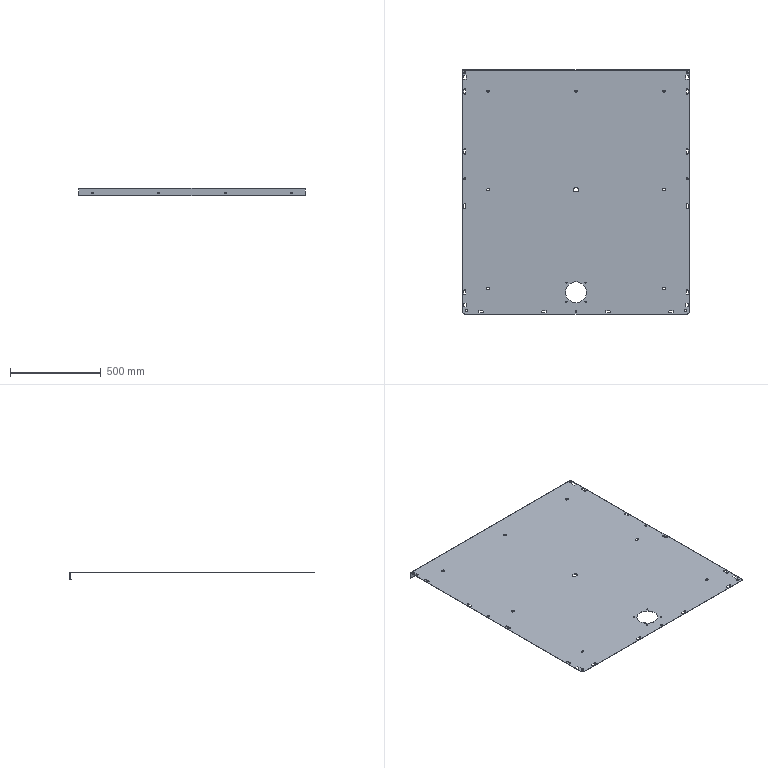Part | SolidWorks | features Cut 6, ICE 4, EdgeFlange 2, Fillet 1, FlatPattern 1, SMBaseFlange 1, SheetMetal 1 | 1 solid | 172 faces | box 1250 x 1345 x 39.5 mm | volume 2576093 mm3 | cylinder 90 | plane 82 | commonest cylinder face diameters 10 x34 11 x25 5.9 x8 10.5 x8 12.8 x4 20 x3